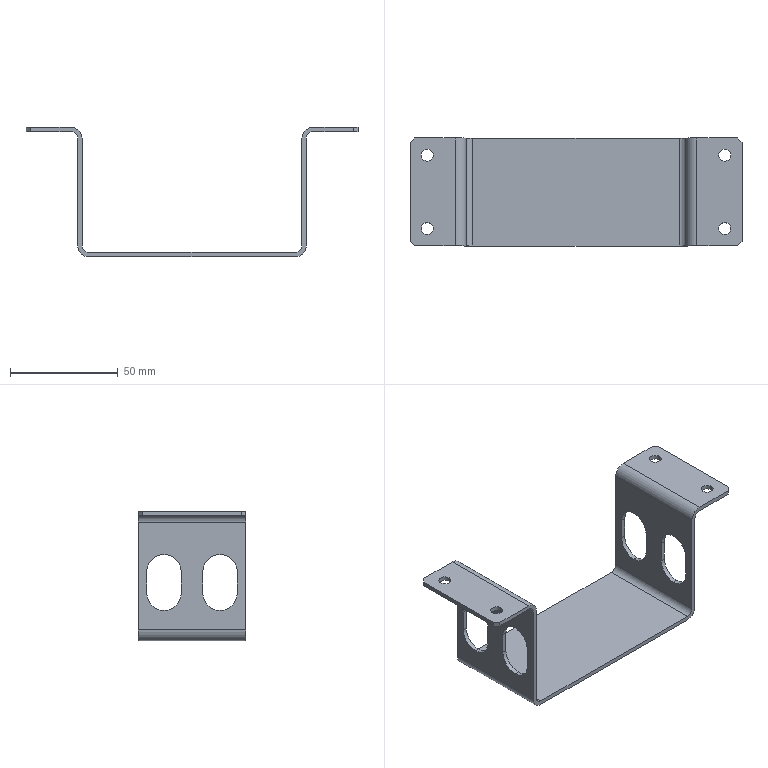Part | STEP file | Three-control-box air switch baffle | 1 solid | 54 faces | box 154 x 50 x 60 mm | volume 23219 mm3 | cylinder 28 | plane 26 | commonest cylinder face diameters 16 x12 5.5 x8 6 x4 10 x4